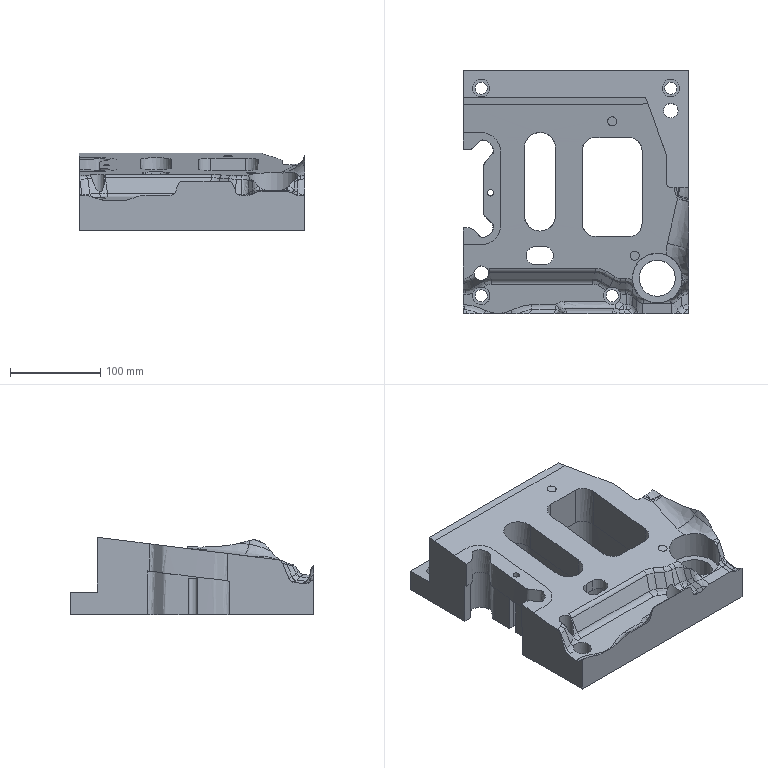Part | NX | features solid 2 | 1 solid | 185 faces | box 250.006 x 270.004 x 85.748 mm | volume 2844726 mm3 | spline 139 | plane 28 | cylinder 18 | commonest cylinder face diameters 13.5 x4 19.5 x4 10 x2 16 x2 20 x2 7 x1